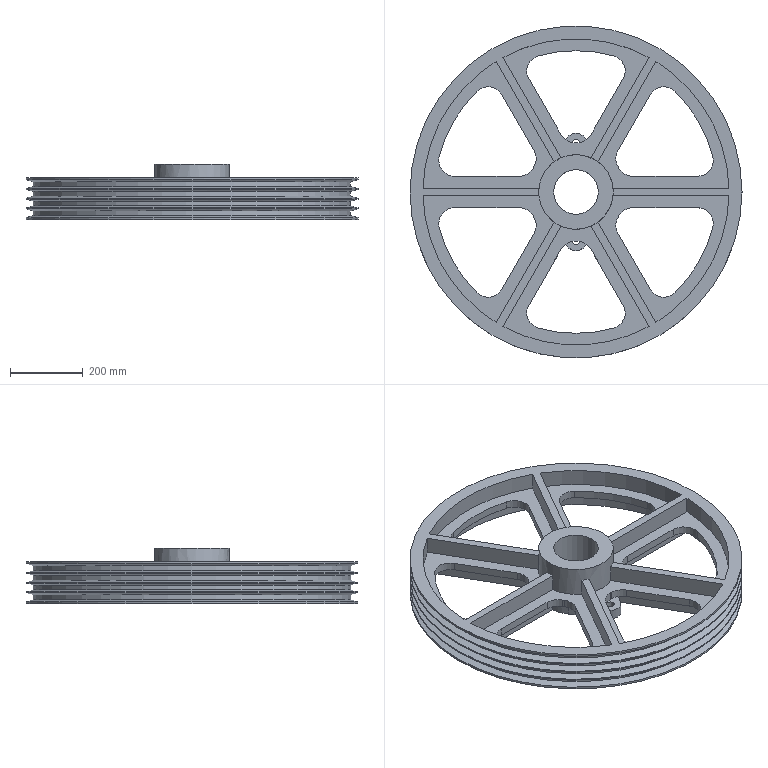Part | NX | features BREP 1, SCALE 1, SPLIT BODY 1, UNITE 1 | 1 solid | 150 faces | box 915.408 x 915.408 x 151.725 mm | volume 20057107 mm3 | cylinder 77 | plane 65 | cone 8 | commonest cylinder face diameters 86.7 x30 843.88 x12 205.912 x7 270.938 x6 778.855 x6 915.408 x5